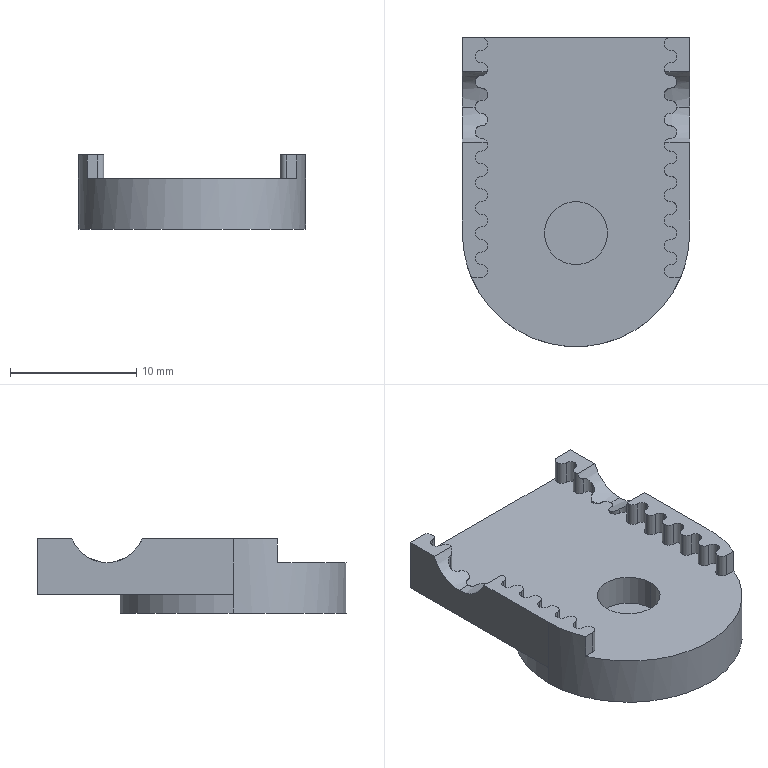Part | SolidWorks | features BaseBody 1 | 1 solid | 79 faces | box 18 x 24.5 x 5.9 mm | volume 1432 mm3 | cylinder 66 | plane 13 | commonest cylinder face diameters 1 x58 6 x4 5 x2 18 x2